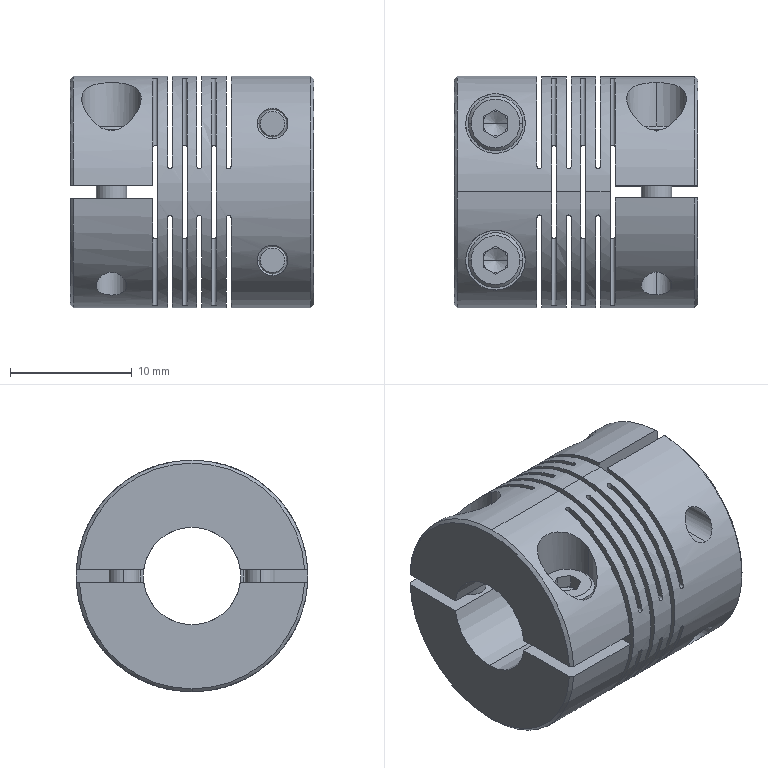Part | SolidWorks | features AEMSimFeature 1 | 5 solids | 232 faces | box 20 x 19 x 19 mm | volume 3812 mm3 | plane 100 | cylinder 87 | cone 45 | commonest cylinder face diameters 0.4 x30 2.5 x24 2.013 x8 4.5 x8 4.9 x8 8 x5